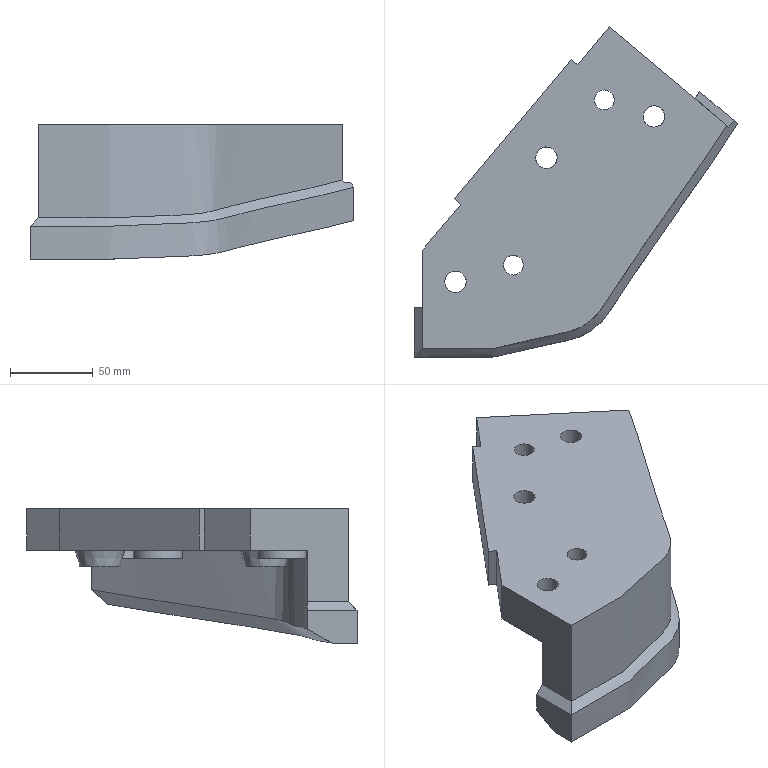Part | NX | features solid 2 | 1 solid | 38 faces | box 195.734 x 199.607 x 81.302 mm | volume 814475 mm3 | plane 20 | cylinder 10 | spline 6 | cone 2 | commonest cylinder face diameters 13 x5 30 x3 12 x2